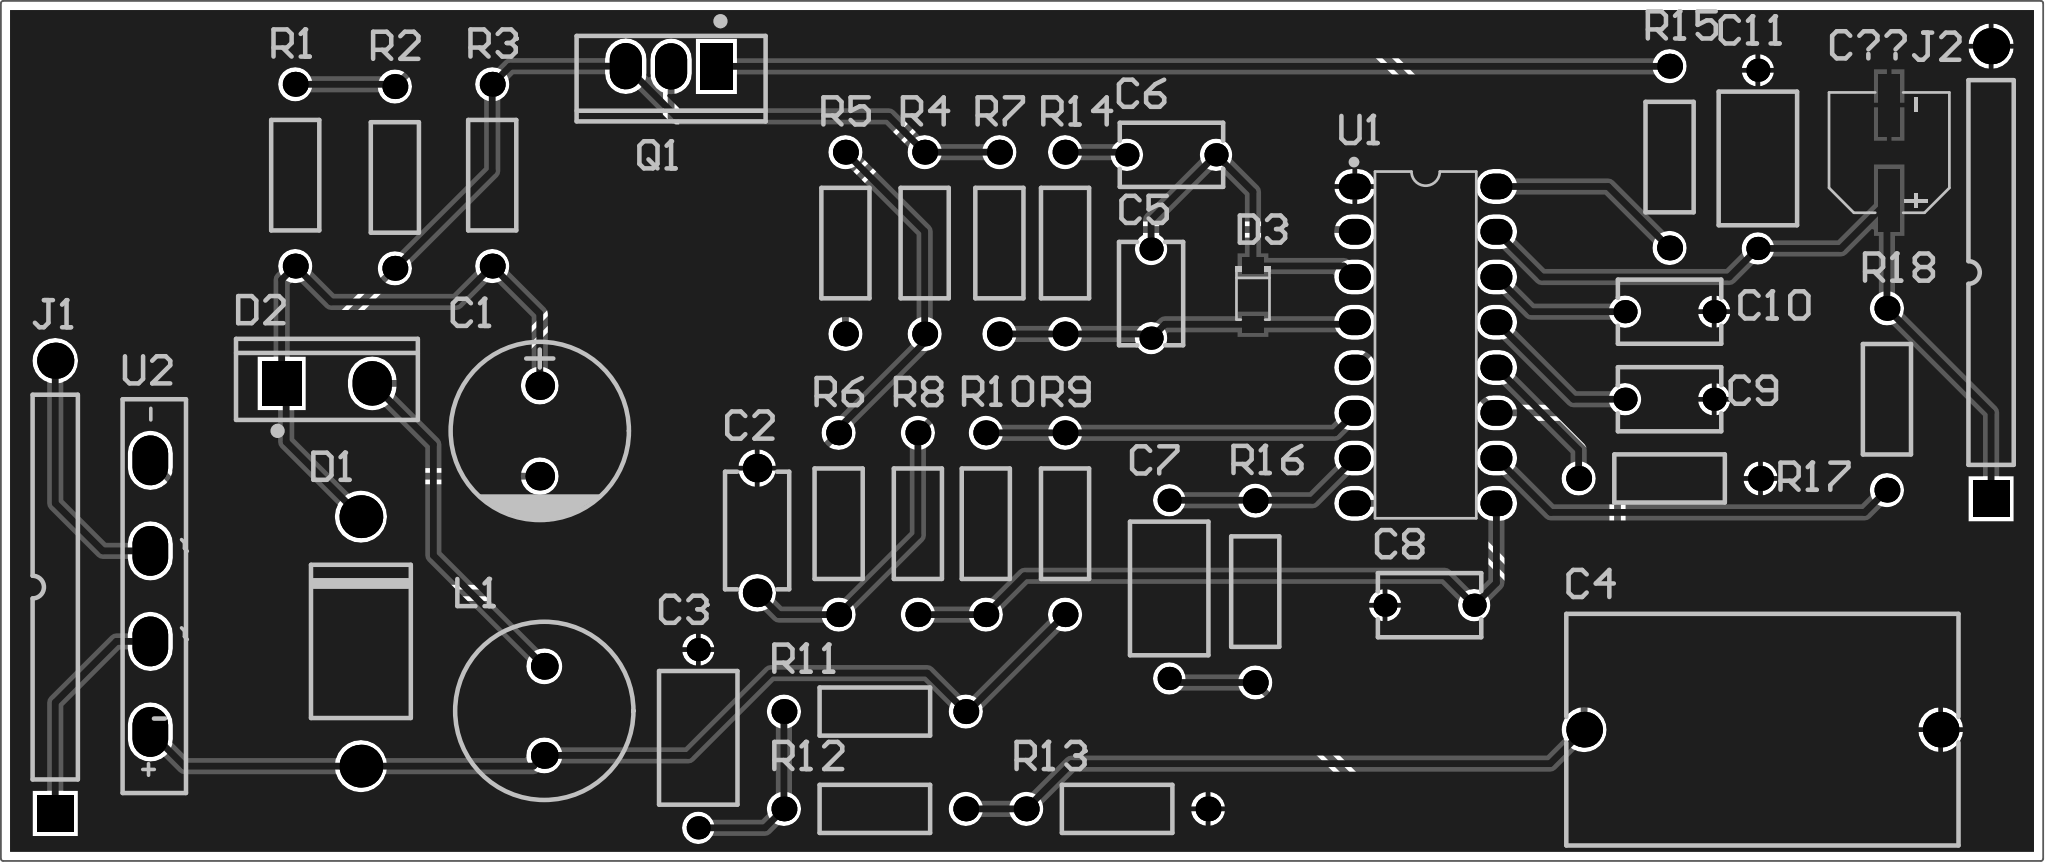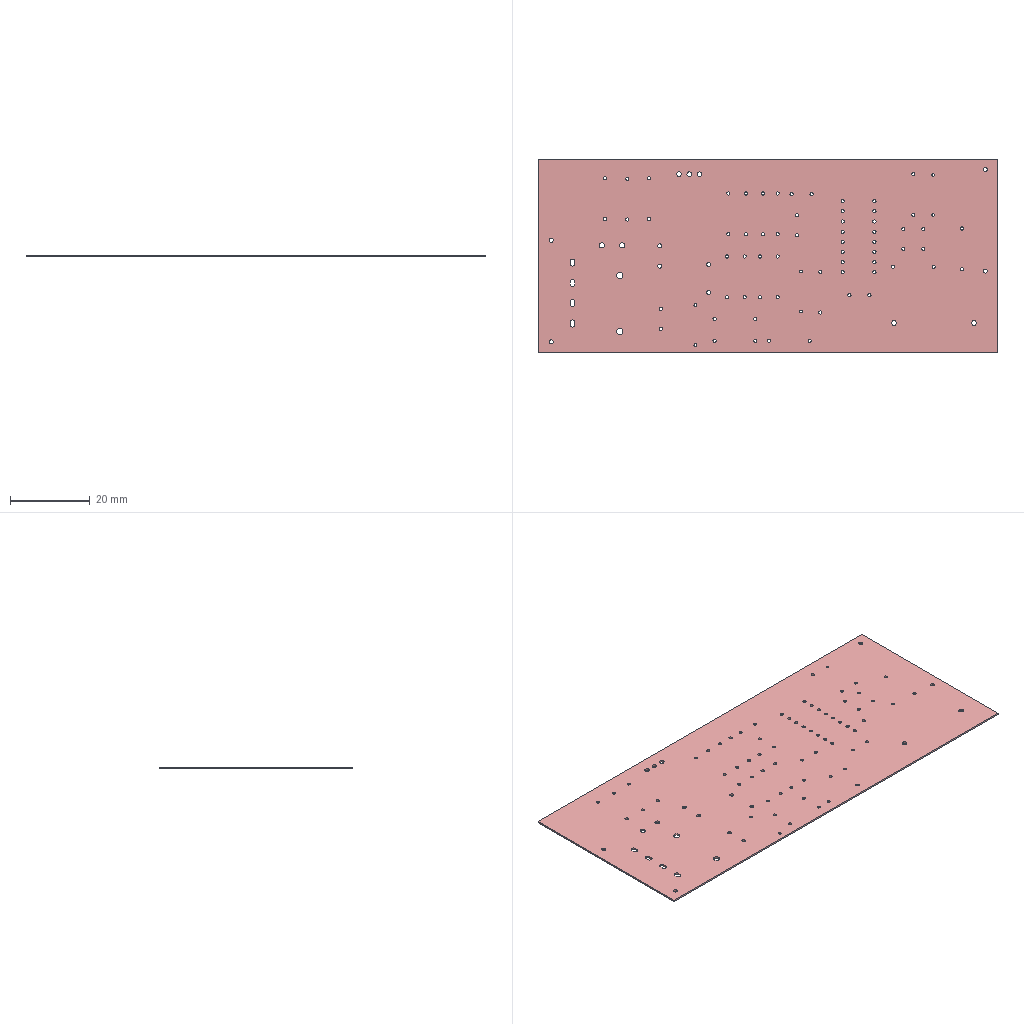Circuit board layout | Altium Designer | box 114.6 x 48.3 x 0.4 mm
Part placement:
Designator,Comment,Layer,Footprint,Center-X(mm),Center-Y(mm),Rotation
C1,LKME1402A101MF,TopLayer,CAP-TH_BD10.0-P5.00-D1.0-FD,93.599,61.722,270
C2,KJKF222M2FF7035A075E,TopLayer,CAP-TH_L6.5-W3.5-P7.50-D1.0,105.791,56.134,270
C3,KY1102M400VAC70Y10093,TopLayer,CAP-TH_L7.5-W4.5-P10.00-D0.6,102.489,44.45,270
C4,CBB21-400V/255JP20,TopLayer,CAP-TH_L22.0-W12.5-P20.00-D0.7-FD,162.179,44.958,180
C5,178MU0002,TopLayer,CAP-TH_L5.8-W3.6-P5.0-D0.6,127.889,69.429,90
C6,178MU0002,TopLayer,CAP-TH_L5.8-W3.6-P5.0-D0.6,129.032,77.216,180
C7,KY1102M400VAC70Y10093,TopLayer,CAP-TH_L7.5-W4.5-P10.00-D0.6,128.905,52.832,270
C8,178MU0002,TopLayer,CAP-TH_L5.8-W3.6-P5.0-D0.6,143.51,51.943,360
C9,178MU0002,TopLayer,CAP-TH_L5.8-W3.6-P5.0-D0.6,156.972,63.5,360
C10,178MU0002,TopLayer,CAP-TH_L5.8-W3.6-P5.0-D0.6,156.972,68.413,360
C11,KY1102M400VAC70Y10093,TopLayer,CAP-TH_L7.5-W4.5-P10.00-D0.6,161.925,76.962,270
C??,RVE100UF35V67RV0072,TopLayer,CAP-SMD_BD6.3-L6.6-W6.6-LS7.6-FD-1,169.291,77.34,90
D1,1N5406_C5338388,TopLayer,DO-27_BD5.2-L8.9-P12.90-D1.5-RD,83.566,49.911,270
D2,GC3D10060A,TopLayer,TO-220-2_L10.2-W4.5-P5.08-L-A,81.661,64.389,360
D3,BZT52C8V2_C19077406,TopLayer,SOD-123_L2.7-W1.6-LS3.7-RD,133.604,69.342,270
J1,HOLE,TopLayer,DIP2,66.421,52.959,90
J2,HOLE,TopLayer,DIP2,175.006,70.612,90
L1,XR8*10-101K-L,TopLayer,IND-TH_BD10.0-P5.00-D0.6,93.853,46.014,90
Q1,IRF530NPBF,TopLayer,TO-220-3_L10.0-W4.5-P2.54-L,100.965,82.184,180
R1,MF1/4W-100K±1%-OT26,TopLayer,RES-TH_BD2.7-L6.2-P10.20-D0.4,79.883,76.073,270
R2,MF1/4W-100K±1%-OT26,TopLayer,RES-TH_BD2.7-L6.2-P10.20-D0.4,85.471,75.946,90
R3,MF1/4W-100K±1%-OT26,TopLayer,RES-TH_BD2.7-L6.2-P10.20-D0.4,90.932,76.073,270
R4,MF1/4W-100K±1%-OT26,TopLayer,RES-TH_BD2.7-L6.2-P10.20-D0.4,115.189,72.263,90
R5,MF1/4W-100K±1%-OT26,TopLayer,RES-TH_BD2.7-L6.2-P10.20-D0.4,110.744,72.263,90
R6,MF1/4W-100K±1%-OT26,TopLayer,RES-TH_BD2.7-L6.2-P10.20-D0.4,110.363,56.515,90
R7,MF1/4W-100K±1%-OT26,TopLayer,RES-TH_BD2.7-L6.2-P10.20-D0.4,119.38,72.263,90
R8,MF1/4W-100K±1%-OT26,TopLayer,RES-TH_BD2.7-L6.2-P10.20-D0.4,114.808,56.515,90
R9,MF1/4W-100K±1%-OT26,TopLayer,RES-TH_BD2.7-L6.2-P10.20-D0.4,123.063,56.515,270
R10,MF1/4W-100K±1%-OT26,TopLayer,RES-TH_BD2.7-L6.2-P10.20-D0.4,118.618,56.515,270
R11,MF1/4W-100K±1%-OT26,TopLayer,RES-TH_BD2.7-L6.2-P10.20-D0.4,112.395,45.974,360
R12,MF1/4W-100K±1%-OT26,TopLayer,RES-TH_BD2.7-L6.2-P10.20-D0.4,112.395,40.513,360
R13,MF1/4W-100K±1%-OT26,TopLayer,RES-TH_BD2.7-L6.2-P10.20-D0.4,125.984,40.513,180
R14,MF1/4W-100K±1%-OT26,TopLayer,RES-TH_BD2.7-L6.2-P10.20-D0.4,123.063,72.263,90
R15,MF1/4W-100K±1%-OT26,TopLayer,RES-TH_BD2.7-L6.2-P10.20-D0.4,156.972,77.089,270
R16,MF1/4W-100K±1%-OT26,TopLayer,RES-TH_BD2.7-L6.2-P10.20-D0.4,133.731,52.705,270
R17,MF1/4W-100K±1%-OT26,TopLayer,RES-TH_BD2.7-L6.2-P10.20-D0.4,156.972,59.055,360
R18,MF1/4W-100K±1%-OT26,TopLayer,RES-TH_BD2.7-L6.2-P10.20-D0.4,169.164,63.5,90
U1,UC3854N,TopLayer,PDIP-16_L19.3-W6.4-P2.54-LS7.94-BL,143.289,66.548,270
U2,GBU8K,TopLayer,GBU_4P-L22.0-W3.5-P5.08-GBU4K,71.755,52.451,270